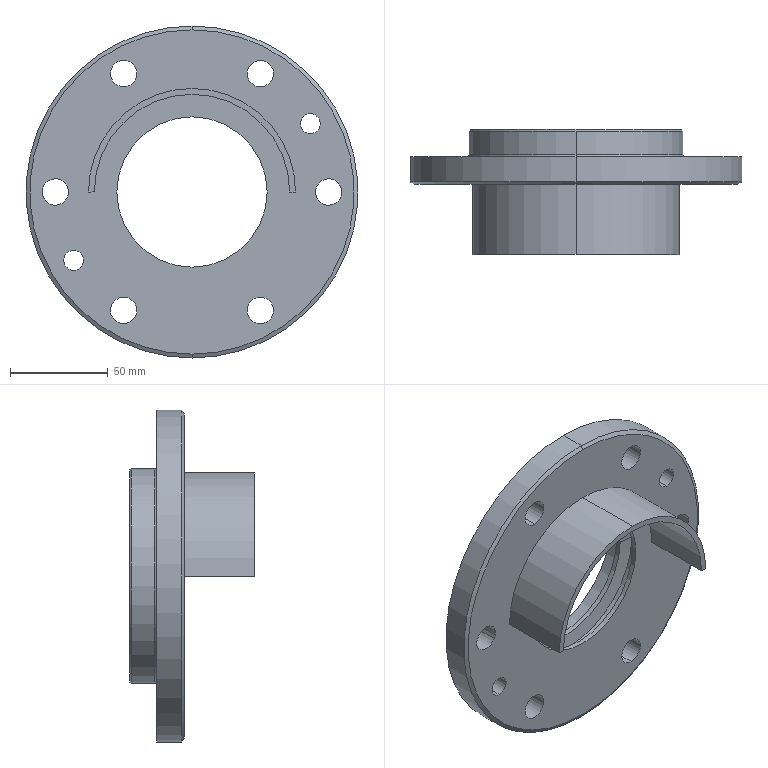Part | SolidWorks | features ICE 3, Chamfer 2, Fillet 2, CirPattern 1, Extrusion 1, HoleWzd 1, RevCut 1 | 1 solid | 51 faces | box 170 x 64 x 170 mm | volume 268447 mm3 | cylinder 32 | cone 8 | plane 7 | torus 4 | commonest cylinder face diameters 13.5 x12 10.2 x4 77 x4 92 x2 98 x2 100 x2
STEP:
#1=CARTESIAN_POINT('',(60.622,14.,29.9));
#2=VERTEX_POINT('',#1);
#3=CARTESIAN_POINT('',(60.622,14.,40.1));
#4=VERTEX_POINT('',#3);
#5=CARTESIAN_POINT('',(60.622,14.,35.));
#6=DIRECTION('',(0.,1.,0.));
#7=DIRECTION('',(0.,0.,1.));
#8=AXIS2_PLACEMENT_3D('',#5,#6,#7);
#9=CIRCLE('',#8,5.1);
#10=EDGE_CURVE('',#2,#4,#9,.T.);
#11=ORIENTED_EDGE('',*,*,#10,.T.);
#12=CARTESIAN_POINT('',(60.622,0.,40.1));
#13=VERTEX_POINT('',#12);
#14=CARTESIAN_POINT('',(60.622,0.,40.1));
#15=DIRECTION('',(0.,-1.,0.));
#16=VECTOR('',#15,1000.);
#17=LINE('',#14,#16);
#18=EDGE_CURVE('',#4,#13,#17,.T.);
#19=ORIENTED_EDGE('',*,*,#18,.T.);
#20=CARTESIAN_POINT('',(60.622,0.,29.9));
#21=VERTEX_POINT('',#20);
#22=CARTESIAN_POINT('',(60.622,0.,35.));
#23=DIRECTION('',(0.,-1.,0.));
#24=DIRECTION('',(0.,0.,-1.));
#25=AXIS2_PLACEMENT_3D('',#22,#23,#24);
#26=CIRCLE('',#25,5.1);
#27=EDGE_CURVE('',#13,#21,#26,.T.);
#28=ORIENTED_EDGE('',*,*,#27,.T.);
#29=CARTESIAN_POINT('',(60.622,0.,29.9));
#30=DIRECTION('',(0.,-1.,0.));
#31=VECTOR('',#30,1000.);
#32=LINE('',#29,#31);
#33=EDGE_CURVE('',#2,#21,#32,.T.);
#34=ORIENTED_EDGE('',*,*,#33,.F.);
#35=EDGE_LOOP('',(#11,#19,#28,#34));
#36=FACE_OUTER_BOUND('',#35,.T.);
#37=CARTESIAN_POINT('',(60.622,0.,35.));
#38=DIRECTION('',(0.,-1.,0.));
#39=DIRECTION('',(0.,0.,-1.));
#40=AXIS2_PLACEMENT_3D('',#37,#38,#39);
#41=CYLINDRICAL_SURFACE('',#40,5.1);
#42=ADVANCED_FACE('',(#36),#41,.F.);
#43=CARTESIAN_POINT('',(-60.622,14.,-40.1));
#44=VERTEX_POINT('',#43);
#45=CARTESIAN_POINT('',(-60.622,14.,-29.9));
#46=VERTEX_POINT('',#45);
#47=CARTESIAN_POINT('',(-60.622,14.,-35.));
#48=DIRECTION('',(0.,1.,0.));
#49=DIRECTION('',(0.,0.,1.));
#50=AXIS2_PLACEMENT_3D('',#47,#48,#49);
#51=CIRCLE('',#50,5.1);
#52=EDGE_CURVE('',#44,#46,#51,.T.);
#53=ORIENTED_EDGE('',*,*,#52,.T.);
#54=CARTESIAN_POINT('',(-60.622,0.,-29.9));
#55=VERTEX_POINT('',#54);
#56=CARTESIAN_POINT('',(-60.622,0.,-29.9));
#57=DIRECTION('',(0.,-1.,0.));
#58=VECTOR('',#57,1000.);
#59=LINE('',#56,#58);
#60=EDGE_CURVE('',#46,#55,#59,.T.);
#61=ORIENTED_EDGE('',*,*,#60,.T.);
#62=CARTESIAN_POINT('',(-60.622,0.,-40.1));
#63=VERTEX_POINT('',#62);
#64=CARTESIAN_POINT('',(-60.622,0.,-35.));
#65=DIRECTION('',(0.,-1.,0.));
#66=DIRECTION('',(0.,0.,-1.));
#67=AXIS2_PLACEMENT_3D('',#64,#65,#66);
#68=CIRCLE('',#67,5.1);
#69=EDGE_CURVE('',#55,#63,#68,.T.);
#70=ORIENTED_EDGE('',*,*,#69,.T.);
#71=CARTESIAN_POINT('',(-60.622,0.,-40.1));
#72=DIRECTION('',(0.,-1.,0.));
#73=VECTOR('',#72,1000.);
#74=LINE('',#71,#73);
#75=EDGE_CURVE('',#44,#63,#74,.T.);
#76=ORIENTED_EDGE('',*,*,#75,.F.);
#77=EDGE_LOOP('',(#53,#61,#70,#76));
#78=FACE_OUTER_BOUND('',#77,.T.);
#79=CARTESIAN_POINT('',(-60.622,0.,-35.));
#80=DIRECTION('',(0.,-1.,0.));
#81=DIRECTION('',(0.,0.,-1.));
#82=AXIS2_PLACEMENT_3D('',#79,#80,#81);
#83=CYLINDRICAL_SURFACE('',#82,5.1);
#84=ADVANCED_FACE('',(#78),#83,.F.);
#85=CARTESIAN_POINT('',(29.154,14.,57.247));
#86=VERTEX_POINT('',#85);
#87=CARTESIAN_POINT('',(40.846,14.,63.997));
#88=VERTEX_POINT('',#87);
#89=CARTESIAN_POINT('',(35.,14.,60.622));
#90=DIRECTION('',(0.,1.,0.));
#91=DIRECTION('',(0.866,0.,0.5));
#92=AXIS2_PLACEMENT_3D('',#89,#90,#91);
#93=CIRCLE('',#92,6.75);
#94=EDGE_CURVE('',#86,#88,#93,.T.);
#95=ORIENTED_EDGE('',*,*,#94,.T.);
#96=CARTESIAN_POINT('',(40.846,0.,63.997));
#97=VERTEX_POINT('',#96);
#98=CARTESIAN_POINT('',(40.846,28.,63.997));
#99=DIRECTION('',(0.,-1.,0.));
#100=VECTOR('',#99,1000.);
#101=LINE('',#98,#100);
#102=EDGE_CURVE('',#88,#97,#101,.T.);
#103=ORIENTED_EDGE('',*,*,#102,.T.);
#104=CARTESIAN_POINT('',(29.154,0.,57.247));
#105=VERTEX_POINT('',#104);
#106=CARTESIAN_POINT('',(35.,0.,60.622));
#107=DIRECTION('',(0.,-1.,0.));
#108=DIRECTION('',(-0.866,0.,-0.5));
#109=AXIS2_PLACEMENT_3D('',#106,#107,#108);
#110=CIRCLE('',#109,6.75);
#111=EDGE_CURVE('',#97,#105,#110,.T.);
#112=ORIENTED_EDGE('',*,*,#111,.T.);
#113=CARTESIAN_POINT('',(29.154,28.,57.247));
#114=DIRECTION('',(0.,-1.,0.));
#115=VECTOR('',#114,1000.);
#116=LINE('',#113,#115);
#117=EDGE_CURVE('',#86,#105,#116,.T.);
#118=ORIENTED_EDGE('',*,*,#117,.F.);
#119=EDGE_LOOP('',(#95,#103,#112,#118));
#120=FACE_OUTER_BOUND('',#119,.T.);
#121=CARTESIAN_POINT('',(35.,28.,60.622));
#122=DIRECTION('',(0.,-1.,0.));
#123=DIRECTION('',(-0.866,0.,-0.5));
#124=AXIS2_PLACEMENT_3D('',#121,#122,#123);
#125=CYLINDRICAL_SURFACE('',#124,6.75);
#126=ADVANCED_FACE('',(#120),#125,.F.);
#127=CARTESIAN_POINT('',(64.154,14.,3.375));
#128=VERTEX_POINT('',#127);
#129=CARTESIAN_POINT('',(75.846,14.,-3.375));
#130=VERTEX_POINT('',#129);
#131=CARTESIAN_POINT('',(70.,14.,0.));
#132=DIRECTION('',(0.,1.,0.));
#133=DIRECTION('',(0.866,0.,-0.5));
#134=AXIS2_PLACEMENT_3D('',#131,#132,#133);
#135=CIRCLE('',#134,6.75);
#136=EDGE_CURVE('',#128,#130,#135,.T.);
#137=ORIENTED_EDGE('',*,*,#136,.T.);
#138=CARTESIAN_POINT('',(75.846,0.,-3.375));
#139=VERTEX_POINT('',#138);
#140=CARTESIAN_POINT('',(75.846,28.,-3.375));
#141=DIRECTION('',(0.,-1.,0.));
#142=VECTOR('',#141,1000.);
#143=LINE('',#140,#142);
#144=EDGE_CURVE('',#130,#139,#143,.T.);
#145=ORIENTED_EDGE('',*,*,#144,.T.);
#146=CARTESIAN_POINT('',(64.154,0.,3.375));
#147=VERTEX_POINT('',#146);
#148=CARTESIAN_POINT('',(70.,0.,0.));
#149=DIRECTION('',(0.,-1.,0.));
#150=DIRECTION('',(-0.866,0.,0.5));
#151=AXIS2_PLACEMENT_3D('',#148,#149,#150);
#152=CIRCLE('',#151,6.75);
#153=EDGE_CURVE('',#139,#147,#152,.T.);
#154=ORIENTED_EDGE('',*,*,#153,.T.);
#155=CARTESIAN_POINT('',(64.154,28.,3.375));
#156=DIRECTION('',(0.,-1.,0.));
#157=VECTOR('',#156,1000.);
#158=LINE('',#155,#157);
#159=EDGE_CURVE('',#128,#147,#158,.T.);
#160=ORIENTED_EDGE('',*,*,#159,.F.);
#161=EDGE_LOOP('',(#137,#145,#154,#160));
#162=FACE_OUTER_BOUND('',#161,.T.);
#163=CARTESIAN_POINT('',(70.,28.,0.));
#164=DIRECTION('',(0.,-1.,0.));
#165=DIRECTION('',(-0.866,0.,0.5));
#166=AXIS2_PLACEMENT_3D('',#163,#164,#165);
#167=CYLINDRICAL_SURFACE('',#166,6.75);
#168=ADVANCED_FACE('',(#162),#167,.F.);
#169=CARTESIAN_POINT('',(35.,14.,-53.872));
#170=VERTEX_POINT('',#169);
#171=CARTESIAN_POINT('',(35.,14.,-67.372));
#172=VERTEX_POINT('',#171);
#173=CARTESIAN_POINT('',(35.,14.,-60.622));
#174=DIRECTION('',(0.,1.,0.));
#175=DIRECTION('',(0.,0.,-1.));
#176=AXIS2_PLACEMENT_3D('',#173,#174,#175);
#177=CIRCLE('',#176,6.75);
#178=EDGE_CURVE('',#170,#172,#177,.T.);
#179=ORIENTED_EDGE('',*,*,#178,.T.);
#180=CARTESIAN_POINT('',(35.,0.,-67.372));
#181=VERTEX_POINT('',#180);
#182=CARTESIAN_POINT('',(35.,28.,-67.372));
#183=DIRECTION('',(0.,-1.,0.));
#184=VECTOR('',#183,1000.);
#185=LINE('',#182,#184);
#186=EDGE_CURVE('',#172,#181,#185,.T.);
#187=ORIENTED_EDGE('',*,*,#186,.T.);
#188=CARTESIAN_POINT('',(35.,0.,-53.872));
#189=VERTEX_POINT('',#188);
#190=CARTESIAN_POINT('',(35.,0.,-60.622));
#191=DIRECTION('',(0.,-1.,0.));
#192=DIRECTION('',(0.,0.,1.));
#193=AXIS2_PLACEMENT_3D('',#190,#191,#192);
#194=CIRCLE('',#193,6.75);
#195=EDGE_CURVE('',#181,#189,#194,.T.);
#196=ORIENTED_EDGE('',*,*,#195,.T.);
#197=CARTESIAN_POINT('',(35.,28.,-53.872));
#198=DIRECTION('',(0.,-1.,0.));
#199=VECTOR('',#198,1000.);
#200=LINE('',#197,#199);
#201=EDGE_CURVE('',#170,#189,#200,.T.);
#202=ORIENTED_EDGE('',*,*,#201,.F.);
#203=EDGE_LOOP('',(#179,#187,#196,#202));
#204=FACE_OUTER_BOUND('',#203,.T.);
#205=CARTESIAN_POINT('',(35.,28.,-60.622));
#206=DIRECTION('',(0.,-1.,0.));
#207=DIRECTION('',(0.,0.,1.));
#208=AXIS2_PLACEMENT_3D('',#205,#206,#207);
#209=CYLINDRICAL_SURFACE('',#208,6.75);
#210=ADVANCED_FACE('',(#204),#209,.F.);
#211=CARTESIAN_POINT('',(-29.154,14.,-57.247));
#212=VERTEX_POINT('',#211);
#213=CARTESIAN_POINT('',(-40.846,14.,-63.997));
#214=VERTEX_POINT('',#213);
#215=CARTESIAN_POINT('',(-35.,14.,-60.622));
#216=DIRECTION('',(0.,1.,0.));
#217=DIRECTION('',(-0.866,0.,-0.5));
#218=AXIS2_PLACEMENT_3D('',#215,#216,#217);
#219=CIRCLE('',#218,6.75);
#220=EDGE_CURVE('',#212,#214,#219,.T.);
#221=ORIENTED_EDGE('',*,*,#220,.T.);
#222=CARTESIAN_POINT('',(-40.846,0.,-63.997));
#223=VERTEX_POINT('',#222);
#224=CARTESIAN_POINT('',(-40.846,28.,-63.997));
#225=DIRECTION('',(0.,-1.,0.));
#226=VECTOR('',#225,1000.);
#227=LINE('',#224,#226);
#228=EDGE_CURVE('',#214,#223,#227,.T.);
#229=ORIENTED_EDGE('',*,*,#228,.T.);
#230=CARTESIAN_POINT('',(-29.154,0.,-57.247));
#231=VERTEX_POINT('',#230);
#232=CARTESIAN_POINT('',(-35.,0.,-60.622));
#233=DIRECTION('',(0.,-1.,0.));
#234=DIRECTION('',(0.866,0.,0.5));
#235=AXIS2_PLACEMENT_3D('',#232,#233,#234);
#236=CIRCLE('',#235,6.75);
#237=EDGE_CURVE('',#223,#231,#236,.T.);
#238=ORIENTED_EDGE('',*,*,#237,.T.);
#239=CARTESIAN_POINT('',(-29.154,28.,-57.247));
#240=DIRECTION('',(0.,-1.,0.));
#241=VECTOR('',#240,1000.);
#242=LINE('',#239,#241);
#243=EDGE_CURVE('',#212,#231,#242,.T.);
#244=ORIENTED_EDGE('',*,*,#243,.F.);
#245=EDGE_LOOP('',(#221,#229,#238,#244));
#246=FACE_OUTER_BOUND('',#245,.T.);
#247=CARTESIAN_POINT('',(-35.,28.,-60.622));
#248=DIRECTION('',(0.,-1.,0.));
#249=DIRECTION('',(0.866,0.,0.5));
#250=AXIS2_PLACEMENT_3D('',#247,#248,#249);
#251=CYLINDRICAL_SURFACE('',#250,6.75);
#252=ADVANCED_FACE('',(#246),#251,.F.);
#253=CARTESIAN_POINT('',(-64.154,14.,-3.375));
#254=VERTEX_POINT('',#253);
#255=CARTESIAN_POINT('',(-75.846,14.,3.375));
#256=VERTEX_POINT('',#255);
#257=CARTESIAN_POINT('',(-70.,14.,0.));
#258=DIRECTION('',(0.,1.,0.));
#259=DIRECTION('',(-0.866,0.,0.5));
#260=AXIS2_PLACEMENT_3D('',#257,#258,#259);
#261=CIRCLE('',#260,6.75);
#262=EDGE_CURVE('',#254,#256,#261,.T.);
#263=ORIENTED_EDGE('',*,*,#262,.T.);
#264=CARTESIAN_POINT('',(-75.846,0.,3.375));
#265=VERTEX_POINT('',#264);
#266=CARTESIAN_POINT('',(-75.846,28.,3.375));
#267=DIRECTION('',(0.,-1.,0.));
#268=VECTOR('',#267,1000.);
#269=LINE('',#266,#268);
#270=EDGE_CURVE('',#256,#265,#269,.T.);
#271=ORIENTED_EDGE('',*,*,#270,.T.);
#272=CARTESIAN_POINT('',(-64.154,0.,-3.375));
#273=VERTEX_POINT('',#272);
#274=CARTESIAN_POINT('',(-70.,0.,0.));
#275=DIRECTION('',(0.,-1.,0.));
#276=DIRECTION('',(0.866,0.,-0.5));
#277=AXIS2_PLACEMENT_3D('',#274,#275,#276);
#278=CIRCLE('',#277,6.75);
#279=EDGE_CURVE('',#265,#273,#278,.T.);
#280=ORIENTED_EDGE('',*,*,#279,.T.);
#281=CARTESIAN_POINT('',(-64.154,28.,-3.375));
#282=DIRECTION('',(0.,-1.,0.));
#283=VECTOR('',#282,1000.);
#284=LINE('',#281,#283);
#285=EDGE_CURVE('',#254,#273,#284,.T.);
#286=ORIENTED_EDGE('',*,*,#285,.F.);
#287=EDGE_LOOP('',(#263,#271,#280,#286));
#288=FACE_OUTER_BOUND('',#287,.T.);
#289=CARTESIAN_POINT('',(-70.,28.,0.));
#290=DIRECTION('',(0.,-1.,0.));
#291=DIRECTION('',(0.866,0.,-0.5));
#292=AXIS2_PLACEMENT_3D('',#289,#290,#291);
#293=CYLINDRICAL_SURFACE('',#292,6.75);
#294=ADVANCED_FACE('',(#288),#293,.F.);
#295=CARTESIAN_POINT('',(-35.,14.,53.872));
#296=VERTEX_POINT('',#295);
#297=CARTESIAN_POINT('',(-35.,14.,67.372));
#298=VERTEX_POINT('',#297);
#299=CARTESIAN_POINT('',(-35.,14.,60.622));
#300=DIRECTION('',(0.,1.,0.));
#301=DIRECTION('',(0.,0.,1.));
#302=AXIS2_PLACEMENT_3D('',#299,#300,#301);
#303=CIRCLE('',#302,6.75);
#304=EDGE_CURVE('',#296,#298,#303,.T.);
#305=ORIENTED_EDGE('',*,*,#304,.T.);
#306=CARTESIAN_POINT('',(-35.,0.,67.372));
#307=VERTEX_POINT('',#306);
#308=CARTESIAN_POINT('',(-35.,28.,67.372));
#309=DIRECTION('',(0.,-1.,0.));
#310=VECTOR('',#309,1000.);
#311=LINE('',#308,#310);
#312=EDGE_CURVE('',#298,#307,#311,.T.);
#313=ORIENTED_EDGE('',*,*,#312,.T.);
#314=CARTESIAN_POINT('',(-35.,0.,53.872));
#315=VERTEX_POINT('',#314);
#316=CARTESIAN_POINT('',(-35.,0.,60.622));
#317=DIRECTION('',(0.,-1.,0.));
#318=DIRECTION('',(0.,0.,-1.));
#319=AXIS2_PLACEMENT_3D('',#316,#317,#318);
#320=CIRCLE('',#319,6.75);
#321=EDGE_CURVE('',#307,#315,#320,.T.);
#322=ORIENTED_EDGE('',*,*,#321,.T.);
#323=CARTESIAN_POINT('',(-35.,28.,53.872));
#324=DIRECTION('',(0.,-1.,0.));
#325=VECTOR('',#324,1000.);
#326=LINE('',#323,#325);
#327=EDGE_CURVE('',#296,#315,#326,.T.);
#328=ORIENTED_EDGE('',*,*,#327,.F.);
#329=EDGE_LOOP('',(#305,#313,#322,#328));
#330=FACE_OUTER_BOUND('',#329,.T.);
#331=CARTESIAN_POINT('',(-35.,28.,60.622));
#332=DIRECTION('',(0.,-1.,0.));
#333=DIRECTION('',(0.,0.,-1.));
#334=AXIS2_PLACEMENT_3D('',#331,#332,#333);
#335=CYLINDRICAL_SURFACE('',#334,6.75);
#336=ADVANCED_FACE('',(#330),#335,.F.);
#337=CARTESIAN_POINT('',(38.5,11.421,0.));
#338=VERTEX_POINT('',#337);
#339=CARTESIAN_POINT('',(-38.5,11.421,0.));
#340=VERTEX_POINT('',#339);
#341=CARTESIAN_POINT('',(0.,11.421,0.));
#342=DIRECTION('',(0.,1.,0.));
#343=DIRECTION('',(-1.,0.,0.));
#344=AXIS2_PLACEMENT_3D('',#341,#342,#343);
#345=CIRCLE('',#344,38.5);
#346=EDGE_CURVE('',#338,#340,#345,.T.);
#347=ORIENTED_EDGE('',*,*,#346,.F.);
#348=CARTESIAN_POINT('',(38.5,14.,0.));
#349=VERTEX_POINT('',#348);
#350=CARTESIAN_POINT('',(38.5,14.,0.));
#351=DIRECTION('',(0.,1.,0.));
#352=VECTOR('',#351,1000.);
#353=LINE('',#350,#352);
#354=EDGE_CURVE('',#338,#349,#353,.T.);
#355=ORIENTED_EDGE('',*,*,#354,.T.);
#356=CARTESIAN_POINT('',(-38.5,14.,0.));
#357=VERTEX_POINT('',#356);
#358=CARTESIAN_POINT('',(0.,14.,0.));
#359=DIRECTION('',(0.,1.,0.));
#360=DIRECTION('',(-1.,0.,0.));
#361=AXIS2_PLACEMENT_3D('',#358,#359,#360);
#362=CIRCLE('',#361,38.5);
#363=EDGE_CURVE('',#349,#357,#362,.T.);
#364=ORIENTED_EDGE('',*,*,#363,.T.);
#365=CARTESIAN_POINT('',(-38.5,14.,0.));
#366=DIRECTION('',(0.,1.,0.));
#367=VECTOR('',#366,1000.);
#368=LINE('',#365,#367);
#369=EDGE_CURVE('',#340,#357,#368,.T.);
#370=ORIENTED_EDGE('',*,*,#369,.F.);
#371=EDGE_LOOP('',(#347,#355,#364,#370));
#372=FACE_OUTER_BOUND('',#371,.T.);
#373=CARTESIAN_POINT('',(0.,14.,0.));
#374=DIRECTION('',(0.,1.,0.));
#375=DIRECTION('',(-1.,0.,0.));
#376=AXIS2_PLACEMENT_3D('',#373,#374,#375);
#377=CYLINDRICAL_SURFACE('',#376,38.5);
#378=ADVANCED_FACE('',(#372),#377,.F.);
#379=ORIENTED_EDGE('',*,*,#346,.T.);
#380=CARTESIAN_POINT('',(-46.,10.5,0.));
#381=VERTEX_POINT('',#380);
#382=CARTESIAN_POINT('',(-38.5,11.421,0.));
#383=DIRECTION('',(-0.9925,-0.1219,0.));
#384=VECTOR('',#383,1000.);
#385=LINE('',#382,#384);
#386=EDGE_CURVE('',#340,#381,#385,.T.);
#387=ORIENTED_EDGE('',*,*,#386,.T.);
#388=CARTESIAN_POINT('',(46.,10.5,0.));
#389=VERTEX_POINT('',#388);
#390=CARTESIAN_POINT('',(0.,10.5,0.));
#391=DIRECTION('',(0.,1.,0.));
#392=DIRECTION('',(-1.,0.,0.));
#393=AXIS2_PLACEMENT_3D('',#390,#391,#392);
#394=CIRCLE('',#393,46.);
#395=EDGE_CURVE('',#389,#381,#394,.T.);
#396=ORIENTED_EDGE('',*,*,#395,.F.);
#397=CARTESIAN_POINT('',(38.5,11.421,0.));
#398=DIRECTION('',(0.9925,-0.1219,0.));
#399=VECTOR('',#398,1000.);
#400=LINE('',#397,#399);
#401=EDGE_CURVE('',#338,#389,#400,.T.);
#402=ORIENTED_EDGE('',*,*,#401,.F.);
#403=EDGE_LOOP('',(#379,#387,#396,#402));
#404=FACE_OUTER_BOUND('',#403,.T.);
#405=CARTESIAN_POINT('',(0.,11.421,0.));
#406=DIRECTION('',(0.,-1.,0.));
#407=DIRECTION('',(1.,0.,0.));
#408=AXIS2_PLACEMENT_3D('',#405,#406,#407);
#409=CONICAL_SURFACE('',#408,38.5,1.449);
#410=ADVANCED_FACE('',(#404),#409,.F.);
#411=CARTESIAN_POINT('',(46.,3.5,0.));
#412=VERTEX_POINT('',#411);
#413=CARTESIAN_POINT('',(-46.,3.5,0.));
#414=VERTEX_POINT('',#413);
#415=CARTESIAN_POINT('',(0.,3.5,0.));
#416=DIRECTION('',(0.,1.,0.));
#417=DIRECTION('',(-1.,0.,0.));
#418=AXIS2_PLACEMENT_3D('',#415,#416,#417);
#419=CIRCLE('',#418,46.);
#420=EDGE_CURVE('',#412,#414,#419,.T.);
#421=ORIENTED_EDGE('',*,*,#420,.F.);
#422=CARTESIAN_POINT('',(46.,14.,0.));
#423=DIRECTION('',(0.,1.,0.));
#424=VECTOR('',#423,1000.);
#425=LINE('',#422,#424);
#426=EDGE_CURVE('',#412,#389,#425,.T.);
#427=ORIENTED_EDGE('',*,*,#426,.T.);
#428=ORIENTED_EDGE('',*,*,#395,.T.);
#429=CARTESIAN_POINT('',(-46.,14.,0.));
#430=DIRECTION('',(0.,1.,0.));
#431=VECTOR('',#430,1000.);
#432=LINE('',#429,#431);
#433=EDGE_CURVE('',#414,#381,#432,.T.);
#434=ORIENTED_EDGE('',*,*,#433,.F.);
#435=EDGE_LOOP('',(#421,#427,#428,#434));
#436=FACE_OUTER_BOUND('',#435,.T.);
#437=CARTESIAN_POINT('',(0.,14.,0.));
#438=DIRECTION('',(0.,1.,0.));
#439=DIRECTION('',(-1.,0.,0.));
#440=AXIS2_PLACEMENT_3D('',#437,#438,#439);
#441=CYLINDRICAL_SURFACE('',#440,46.);
#442=ADVANCED_FACE('',(#436),#441,.F.);
#443=CARTESIAN_POINT('',(38.5,2.579,0.));
#444=VERTEX_POINT('',#443);
#445=CARTESIAN_POINT('',(-38.5,2.579,0.));
#446=VERTEX_POINT('',#445);
#447=CARTESIAN_POINT('',(0.,2.579,0.));
#448=DIRECTION('',(0.,1.,0.));
#449=DIRECTION('',(-1.,0.,0.));
#450=AXIS2_PLACEMENT_3D('',#447,#448,#449);
#451=CIRCLE('',#450,38.5);
#452=EDGE_CURVE('',#444,#446,#451,.T.);
#453=ORIENTED_EDGE('',*,*,#452,.F.);
#454=CARTESIAN_POINT('',(46.,3.5,0.));
#455=DIRECTION('',(0.9925,0.1219,0.));
#456=VECTOR('',#455,1000.);
#457=LINE('',#454,#456);
#458=EDGE_CURVE('',#444,#412,#457,.T.);
#459=ORIENTED_EDGE('',*,*,#458,.T.);
#460=ORIENTED_EDGE('',*,*,#420,.T.);
#461=CARTESIAN_POINT('',(-46.,3.5,0.));
#462=DIRECTION('',(-0.9925,0.1219,0.));
#463=VECTOR('',#462,1000.);
#464=LINE('',#461,#463);
#465=EDGE_CURVE('',#446,#414,#464,.T.);
#466=ORIENTED_EDGE('',*,*,#465,.F.);
#467=EDGE_LOOP('',(#453,#459,#460,#466));
#468=FACE_OUTER_BOUND('',#467,.T.);
#469=CARTESIAN_POINT('',(0.,3.5,0.));
#470=DIRECTION('',(0.,1.,0.));
#471=DIRECTION('',(-1.,0.,0.));
#472=AXIS2_PLACEMENT_3D('',#469,#470,#471);
#473=CONICAL_SURFACE('',#472,46.,1.449);
#474=ADVANCED_FACE('',(#468),#473,.F.);
#475=CARTESIAN_POINT('',(38.5,0.,0.));
#476=VERTEX_POINT('',#475);
#477=CARTESIAN_POINT('',(-38.5,0.,0.));
#478=VERTEX_POINT('',#477);
#479=CARTESIAN_POINT('',(0.,0.,0.));
#480=DIRECTION('',(0.,1.,0.));
#481=DIRECTION('',(-1.,0.,0.));
#482=AXIS2_PLACEMENT_3D('',#479,#480,#481);
#483=CIRCLE('',#482,38.5);
#484=EDGE_CURVE('',#476,#478,#483,.T.);
#485=ORIENTED_EDGE('',*,*,#484,.F.);
#486=CARTESIAN_POINT('',(38.5,14.,0.));
#487=DIRECTION('',(0.,1.,0.));
#488=VECTOR('',#487,1000.);
#489=LINE('',#486,#488);
#490=EDGE_CURVE('',#476,#444,#489,.T.);
#491=ORIENTED_EDGE('',*,*,#490,.T.);
#492=ORIENTED_EDGE('',*,*,#452,.T.);
#493=CARTESIAN_POINT('',(-38.5,14.,0.));
#494=DIRECTION('',(0.,1.,0.));
#495=VECTOR('',#494,1000.);
#496=LINE('',#493,#495);
#497=EDGE_CURVE('',#478,#446,#496,.T.);
#498=ORIENTED_EDGE('',*,*,#497,.F.);
#499=EDGE_LOOP('',(#485,#491,#492,#498));
#500=FACE_OUTER_BOUND('',#499,.T.);
#501=CARTESIAN_POINT('',(0.,14.,0.));
#502=DIRECTION('',(0.,1.,0.));
#503=DIRECTION('',(-1.,0.,0.));
#504=AXIS2_PLACEMENT_3D('',#501,#502,#503);
#505=CYLINDRICAL_SURFACE('',#504,38.5);
#506=ADVANCED_FACE('',(#500),#505,.F.);
#507=CARTESIAN_POINT('',(0.,-36.,50.));
#508=VERTEX_POINT('',#507);
#509=CARTESIAN_POINT('',(50.,-36.,0.));
#510=VERTEX_POINT('',#509);
#511=CARTESIAN_POINT('',(0.,-36.,0.));
#512=DIRECTION('',(0.,1.,0.));
#513=DIRECTION('',(0.,0.,-1.));
#514=AXIS2_PLACEMENT_3D('',#511,#512,#513);
#515=CIRCLE('',#514,50.);
#516=EDGE_CURVE('',#508,#510,#515,.T.);
#517=ORIENTED_EDGE('',*,*,#516,.F.);
#518=CARTESIAN_POINT('',(0.,0.,50.));
#519=VERTEX_POINT('',#518);
#520=CARTESIAN_POINT('',(0.,-36.,50.));
#521=DIRECTION('',(0.,1.,0.));
#522=VECTOR('',#521,1000.);
#523=LINE('',#520,#522);
#524=EDGE_CURVE('',#508,#519,#523,.T.);
#525=ORIENTED_EDGE('',*,*,#524,.T.);
#526=CARTESIAN_POINT('',(50.,0.,0.));
#527=VERTEX_POINT('',#526);
#528=CARTESIAN_POINT('',(0.,0.,0.));
#529=DIRECTION('',(0.,1.,0.));
#530=DIRECTION('',(0.,0.,-1.));
#531=AXIS2_PLACEMENT_3D('',#528,#529,#530);
#532=CIRCLE('',#531,50.);
#533=EDGE_CURVE('',#519,#527,#532,.T.);
#534=ORIENTED_EDGE('',*,*,#533,.T.);
#535=CARTESIAN_POINT('',(50.,-36.,0.));
#536=DIRECTION('',(0.,1.,0.));
#537=VECTOR('',#536,1000.);
#538=LINE('',#535,#537);
#539=EDGE_CURVE('',#510,#527,#538,.T.);
#540=ORIENTED_EDGE('',*,*,#539,.F.);
#541=EDGE_LOOP('',(#517,#525,#534,#540));
#542=FACE_OUTER_BOUND('',#541,.T.);
#543=CARTESIAN_POINT('',(0.,-36.,0.));
#544=DIRECTION('',(0.,1.,0.));
#545=DIRECTION('',(0.,0.,1.));
#546=AXIS2_PLACEMENT_3D('',#543,#544,#545);
#547=CYLINDRICAL_SURFACE('',#546,50.);
#548=ADVANCED_FACE('',(#542),#547,.F.);
#549=CARTESIAN_POINT('',(0.,-36.,53.));
#550=VERTEX_POINT('',#549);
#551=CARTESIAN_POINT('',(-53.,-36.,0.));
#552=VERTEX_POINT('',#551);
#553=CARTESIAN_POINT('',(0.,-36.,0.));
#554=DIRECTION('',(0.,-1.,0.));
#555=DIRECTION('',(0.,0.,-1.));
#556=AXIS2_PLACEMENT_3D('',#553,#554,#555);
#557=CIRCLE('',#556,53.);
#558=EDGE_CURVE('',#550,#552,#557,.T.);
#559=ORIENTED_EDGE('',*,*,#558,.F.);
#560=CARTESIAN_POINT('',(0.,0.,53.));
#561=VERTEX_POINT('',#560);
#562=CARTESIAN_POINT('',(0.,-36.,53.));
#563=DIRECTION('',(0.,1.,0.));
#564=VECTOR('',#563,1000.);
#565=LINE('',#562,#564);
#566=EDGE_CURVE('',#550,#561,#565,.T.);
#567=ORIENTED_EDGE('',*,*,#566,.T.);
#568=CARTESIAN_POINT('',(-53.,0.,0.));
#569=VERTEX_POINT('',#568);
#570=CARTESIAN_POINT('',(0.,0.,0.));
#571=DIRECTION('',(0.,-1.,0.));
#572=DIRECTION('',(0.,0.,-1.));
#573=AXIS2_PLACEMENT_3D('',#570,#571,#572);
#574=CIRCLE('',#573,53.);
#575=EDGE_CURVE('',#561,#569,#574,.T.);
#576=ORIENTED_EDGE('',*,*,#575,.T.);
#577=CARTESIAN_POINT('',(-53.,-36.,0.));
#578=DIRECTION('',(0.,1.,0.));
#579=VECTOR('',#578,1000.);
#580=LINE('',#577,#579);
#581=EDGE_CURVE('',#552,#569,#580,.T.);
#582=ORIENTED_EDGE('',*,*,#581,.F.);
#583=EDGE_LOOP('',(#559,#567,#576,#582));
#584=FACE_OUTER_BOUND('',#583,.T.);
#585=CARTESIAN_POINT('',(0.,-36.,0.));
#586=DIRECTION('',(0.,1.,0.));
#587=DIRECTION('',(0.,0.,1.));
#588=AXIS2_PLACEMENT_3D('',#585,#586,#587);
#589=CYLINDRICAL_SURFACE('',#588,53.);
#590=ADVANCED_FACE('',(#584),#589,.T.);
#591=CARTESIAN_POINT('',(0.,28.,54.423));
#592=VERTEX_POINT('',#591);
#593=CARTESIAN_POINT('',(0.,28.,-54.423));
#594=VERTEX_POINT('',#593);
#595=CARTESIAN_POINT('',(0.,28.,0.));
#596=DIRECTION('',(0.,1.,0.));
#597=DIRECTION('',(0.,0.,1.));
#598=AXIS2_PLACEMENT_3D('',#595,#596,#597);
#599=CIRCLE('',#598,54.423);
#600=EDGE_CURVE('',#592,#594,#599,.T.);
#601=ORIENTED_EDGE('',*,*,#600,.F.);
#602=CARTESIAN_POINT('',(0.,27.,55.));
#603=VERTEX_POINT('',#602);
#604=CARTESIAN_POINT('',(0.,28.,54.423));
#605=DIRECTION('',(0.,-0.866,0.5));
#606=VECTOR('',#605,1000.);
#607=LINE('',#604,#606);
#608=EDGE_CURVE('',#592,#603,#607,.T.);
#609=ORIENTED_EDGE('',*,*,#608,.T.);
#610=CARTESIAN_POINT('',(0.,27.,-55.));
#611=VERTEX_POINT('',#610);
#612=CARTESIAN_POINT('',(0.,27.,0.));
#613=DIRECTION('',(0.,-1.,0.));
#614=DIRECTION('',(0.,0.,1.));
#615=AXIS2_PLACEMENT_3D('',#612,#613,#614);
#616=CIRCLE('',#615,55.);
#617=EDGE_CURVE('',#611,#603,#616,.T.);
#618=ORIENTED_EDGE('',*,*,#617,.F.);
#619=CARTESIAN_POINT('',(0.,28.,-54.423));
#620=DIRECTION('',(0.,-0.866,-0.5));
#621=VECTOR('',#620,1000.);
#622=LINE('',#619,#621);
#623=EDGE_CURVE('',#594,#611,#622,.T.);
#624=ORIENTED_EDGE('',*,*,#623,.F.);
#625=EDGE_LOOP('',(#601,#609,#618,#624));
#626=FACE_OUTER_BOUND('',#625,.T.);
#627=CARTESIAN_POINT('',(0.,28.,0.));
#628=DIRECTION('',(0.,-1.,0.));
#629=DIRECTION('',(0.,0.,-1.));
#630=AXIS2_PLACEMENT_3D('',#627,#628,#629);
#631=CONICAL_SURFACE('',#630,54.423,0.5236);
#632=ADVANCED_FACE('',(#626),#631,.T.);
#633=CARTESIAN_POINT('',(0.,0.,-83.));
#634=VERTEX_POINT('',#633);
#635=CARTESIAN_POINT('',(0.,0.,83.));
#636=VERTEX_POINT('',#635);
#637=CARTESIAN_POINT('',(0.,0.,0.));
#638=DIRECTION('',(0.,-1.,0.));
#639=DIRECTION('',(0.,0.,1.));
#640=AXIS2_PLACEMENT_3D('',#637,#638,#639);
#641=CIRCLE('',#640,83.);
#642=EDGE_CURVE('',#634,#636,#641,.T.);
#643=ORIENTED_EDGE('',*,*,#642,.F.);
#644=CARTESIAN_POINT('',(0.,1.155,-85.));
#645=VERTEX_POINT('',#644);
#646=CARTESIAN_POINT('',(0.,1.155,-85.));
#647=DIRECTION('',(0.,0.5,-0.866));
#648=VECTOR('',#647,1000.);
#649=LINE('',#646,#648);
#650=EDGE_CURVE('',#634,#645,#649,.T.);
#651=ORIENTED_EDGE('',*,*,#650,.T.);
#652=CARTESIAN_POINT('',(0.,1.155,85.));
#653=VERTEX_POINT('',#652);
#654=CARTESIAN_POINT('',(0.,1.155,0.));
#655=DIRECTION('',(0.,1.,0.));
#656=DIRECTION('',(0.,0.,1.));
#657=AXIS2_PLACEMENT_3D('',#654,#655,#656);
#658=CIRCLE('',#657,85.);
#659=EDGE_CURVE('',#653,#645,#658,.T.);
#660=ORIENTED_EDGE('',*,*,#659,.F.);
#661=CARTESIAN_POINT('',(0.,1.155,85.));
#662=DIRECTION('',(0.,0.5,0.866));
#663=VECTOR('',#662,1000.);
#664=LINE('',#661,#663);
#665=EDGE_CURVE('',#636,#653,#664,.T.);
#666=ORIENTED_EDGE('',*,*,#665,.F.);
#667=EDGE_LOOP('',(#643,#651,#660,#666));
#668=FACE_OUTER_BOUND('',#667,.T.);
#669=CARTESIAN_POINT('',(0.,1.155,0.));
#670=DIRECTION('',(0.,1.,0.));
#671=DIRECTION('',(0.,0.,1.));
#672=AXIS2_PLACEMENT_3D('',#669,#670,#671);
#673=CONICAL_SURFACE('',#672,85.,1.047);
#674=ADVANCED_FACE('',(#668),#673,.T.);
#675=CARTESIAN_POINT('',(0.,15.,-55.));
#676=VERTEX_POINT('',#675);
#677=CARTESIAN_POINT('',(0.,15.,55.));
#678=VERTEX_POINT('',#677);
#679=CARTESIAN_POINT('',(0.,15.,0.));
#680=DIRECTION('',(0.,1.,0.));
#681=DIRECTION('',(0.,0.,1.));
#682=AXIS2_PLACEMENT_3D('',#679,#680,#681);
#683=CIRCLE('',#682,55.);
#684=EDGE_CURVE('',#676,#678,#683,.T.);
#685=ORIENTED_EDGE('',*,*,#684,.F.);
#686=CARTESIAN_POINT('',(0.,14.,-56.));
#687=VERTEX_POINT('',#686);
#688=CARTESIAN_POINT('',(0.,15.,-56.));
#689=DIRECTION('',(1.,0.,0.));
#690=DIRECTION('',(0.,0.,-1.));
#691=AXIS2_PLACEMENT_3D('',#688,#689,#690);
#692=CIRCLE('',#691,1.);
#693=EDGE_CURVE('',#676,#687,#692,.T.);
#694=ORIENTED_EDGE('',*,*,#693,.T.);
#695=CARTESIAN_POINT('',(0.,14.,56.));
#696=VERTEX_POINT('',#695);
#697=CARTESIAN_POINT('',(0.,14.,0.));
#698=DIRECTION('',(0.,-1.,0.));
#699=DIRECTION('',(0.,0.,1.));
#700=AXIS2_PLACEMENT_3D('',#697,#698,#699);
#701=CIRCLE('',#700,56.);
#702=EDGE_CURVE('',#696,#687,#701,.T.);
#703=ORIENTED_EDGE('',*,*,#702,.F.);
#704=CARTESIAN_POINT('',(0.,15.,56.));
#705=DIRECTION('',(-1.,0.,0.));
#706=DIRECTION('',(0.,0.,1.));
#707=AXIS2_PLACEMENT_3D('',#704,#705,#706);
#708=CIRCLE('',#707,1.);
#709=EDGE_CURVE('',#678,#696,#708,.T.);
#710=ORIENTED_EDGE('',*,*,#709,.F.);
#711=EDGE_LOOP('',(#685,#694,#703,#710));
#712=FACE_OUTER_BOUND('',#711,.T.);
#713=CARTESIAN_POINT('',(0.,15.,0.));
#714=DIRECTION('',(0.,1.,0.));
#715=DIRECTION('',(0.,0.,1.));
#716=AXIS2_PLACEMENT_3D('',#713,#714,#715);
#717=TOROIDAL_SURFACE('',#716,56.,1.);
#718=ADVANCED_FACE('',(#712),#717,.F.);
#719=CARTESIAN_POINT('',(0.,14.,-44.));
#720=VERTEX_POINT('',#719);
#721=CARTESIAN_POINT('',(0.,14.,44.));
#722=VERTEX_POINT('',#721);
#723=CARTESIAN_POINT('',(0.,14.,0.));
#724=DIRECTION('',(0.,1.,0.));
#725=DIRECTION('',(0.,0.,1.));
#726=AXIS2_PLACEMENT_3D('',#723,#724,#725);
#727=CIRCLE('',#726,44.);
#728=EDGE_CURVE('',#720,#722,#727,.T.);
#729=ORIENTED_EDGE('',*,*,#728,.F.);
#730=CARTESIAN_POINT('',(0.,19.,-49.));
#731=VERTEX_POINT('',#730);
#732=CARTESIAN_POINT('',(0.,19.,-44.));
#733=DIRECTION('',(1.,0.,0.));
#734=DIRECTION('',(0.,0.,-1.));
#735=AXIS2_PLACEMENT_3D('',#732,#733,#734);
#736=CIRCLE('',#735,5.);
#737=EDGE_CURVE('',#720,#731,#736,.T.);
#738=ORIENTED_EDGE('',*,*,#737,.T.);
#739=CARTESIAN_POINT('',(0.,19.,49.));
#740=VERTEX_POINT('',#739);
#741=CARTESIAN_POINT('',(0.,19.,0.));
#742=DIRECTION('',(0.,-1.,0.));
#743=DIRECTION('',(0.,0.,1.));
#744=AXIS2_PLACEMENT_3D('',#741,#742,#743);
#745=CIRCLE('',#744,49.);
#746=EDGE_CURVE('',#740,#731,#745,.T.);
#747=ORIENTED_EDGE('',*,*,#746,.F.);
#748=CARTESIAN_POINT('',(0.,19.,44.));
#749=DIRECTION('',(-1.,0.,0.));
#750=DIRECTION('',(0.,0.,1.));
#751=AXIS2_PLACEMENT_3D('',#748,#749,#750);
#752=CIRCLE('',#751,5.);
#753=EDGE_CURVE('',#722,#740,#752,.T.);
#754=ORIENTED_EDGE('',*,*,#753,.F.);
#755=EDGE_LOOP('',(#729,#738,#747,#754));
#756=FACE_OUTER_BOUND('',#755,.T.);
#757=CARTESIAN_POINT('',(0.,19.,0.));
#758=DIRECTION('',(0.,1.,0.));
#759=DIRECTION('',(0.,0.,1.));
#760=AXIS2_PLACEMENT_3D('',#757,#758,#759);
#761=TOROIDAL_SURFACE('',#760,44.,5.);
#762=ADVANCED_FACE('',(#756),#761,.F.);
#763=CARTESIAN_POINT('',(0.,28.,-49.));
#764=VERTEX_POINT('',#763);
#765=CARTESIAN_POINT('',(0.,28.,49.));
#766=VERTEX_POINT('',#765);
#767=CARTESIAN_POINT('',(0.,28.,0.));
#768=DIRECTION('',(0.,1.,0.));
#769=DIRECTION('',(0.,0.,1.));
#770=AXIS2_PLACEMENT_3D('',#767,#768,#769);
#771=CIRCLE('',#770,49.);
#772=EDGE_CURVE('',#764,#766,#771,.T.);
#773=ORIENTED_EDGE('',*,*,#772,.T.);
#774=CARTESIAN_POINT('',(0.,28.,49.));
#775=DIRECTION('',(0.,-1.,0.));
#776=VECTOR('',#775,1000.);
#777=LINE('',#774,#776);
#778=EDGE_CURVE('',#766,#740,#777,.T.);
#779=ORIENTED_EDGE('',*,*,#778,.T.);
#780=ORIENTED_EDGE('',*,*,#746,.T.);
#781=CARTESIAN_POINT('',(0.,28.,-49.));
#782=DIRECTION('',(0.,-1.,0.));
#783=VECTOR('',#782,1000.);
#784=LINE('',#781,#783);
#785=EDGE_CURVE('',#764,#731,#784,.T.);
#786=ORIENTED_EDGE('',*,*,#785,.F.);
#787=EDGE_LOOP('',(#773,#779,#780,#786));
#788=FACE_OUTER_BOUND('',#787,.T.);
#789=CARTESIAN_POINT('',(0.,28.,0.));
#790=DIRECTION('',(0.,-1.,0.));
#791=DIRECTION('',(0.,0.,-1.));
#792=AXIS2_PLACEMENT_3D('',#789,#790,#791);
#793=CYLINDRICAL_SURFACE('',#792,49.);
#794=ADVANCED_FACE('',(#788),#793,.F.);
#795=ORIENTED_EDGE('',*,*,#617,.T.);
#796=CARTESIAN_POINT('',(0.,28.,55.));
#797=DIRECTION('',(0.,-1.,0.));
#798=VECTOR('',#797,1000.);
#799=LINE('',#796,#798);
#800=EDGE_CURVE('',#603,#678,#799,.T.);
#801=ORIENTED_EDGE('',*,*,#800,.T.);
#802=CARTESIAN_POINT('',(0.,15.,0.));
#803=DIRECTION('',(0.,1.,0.));
#804=DIRECTION('',(0.,0.,1.));
#805=AXIS2_PLACEMENT_3D('',#802,#803,#804);
#806=CIRCLE('',#805,55.);
#807=EDGE_CURVE('',#678,#676,#806,.T.);
#808=ORIENTED_EDGE('',*,*,#807,.T.);
#809=CARTESIAN_POINT('',(0.,28.,-55.));
#810=DIRECTION('',(0.,-1.,0.));
#811=VECTOR('',#810,1000.);
#812=LINE('',#809,#811);
#813=EDGE_CURVE('',#611,#676,#812,.T.);
#814=ORIENTED_EDGE('',*,*,#813,.F.);
#815=EDGE_LOOP('',(#795,#801,#808,#814));
#816=FACE_OUTER_BOUND('',#815,.T.);
#817=CARTESIAN_POINT('',(0.,28.,0.));
#818=DIRECTION('',(0.,-1.,0.));
#819=DIRECTION('',(0.,0.,-1.));
#820=AXIS2_PLACEMENT_3D('',#817,#818,#819);
#821=CYLINDRICAL_SURFACE('',#820,55.);
#822=ADVANCED_FACE('',(#816),#821,.T.);
#823=CARTESIAN_POINT('',(0.,14.,85.));
#824=VERTEX_POINT('',#823);
#825=CARTESIAN_POINT('',(0.,14.,-85.));
#826=VERTEX_POINT('',#825);
#827=CARTESIAN_POINT('',(0.,14.,0.));
#828=DIRECTION('',(0.,1.,0.));
#829=DIRECTION('',(0.,0.,1.));
#830=AXIS2_PLACEMENT_3D('',#827,#828,#829);
#831=CIRCLE('',#830,85.);
#832=EDGE_CURVE('',#824,#826,#831,.T.);
#833=ORIENTED_EDGE('',*,*,#832,.F.);
#834=CARTESIAN_POINT('',(0.,14.,85.));
#835=DIRECTION('',(0.,-1.,0.));
#836=VECTOR('',#835,1000.);
#837=LINE('',#834,#836);
#838=EDGE_CURVE('',#824,#653,#837,.T.);
#839=ORIENTED_EDGE('',*,*,#838,.T.);
#840=ORIENTED_EDGE('',*,*,#659,.T.);
#841=CARTESIAN_POINT('',(0.,14.,-85.));
#842=DIRECTION('',(0.,-1.,0.));
#843=VECTOR('',#842,1000.);
#844=LINE('',#841,#843);
#845=EDGE_CURVE('',#826,#645,#844,.T.);
#846=ORIENTED_EDGE('',*,*,#845,.F.);
#847=EDGE_LOOP('',(#833,#839,#840,#846));
#848=FACE_OUTER_BOUND('',#847,.T.);
#849=CARTESIAN_POINT('',(0.,14.,0.));
#850=DIRECTION('',(0.,-1.,0.));
#851=DIRECTION('',(0.,0.,-1.));
#852=AXIS2_PLACEMENT_3D('',#849,#850,#851);
#853=CYLINDRICAL_SURFACE('',#852,85.);
#854=ADVANCED_FACE('',(#848),#853,.T.);
#855=CARTESIAN_POINT('',(60.622,0.,35.));
#856=DIRECTION('',(0.,-1.,0.));
#857=DIRECTION('',(0.,0.,-1.));
#858=AXIS2_PLACEMENT_3D('',#855,#856,#857);
#859=CIRCLE('',#858,5.1);
#860=EDGE_CURVE('',#21,#13,#859,.T.);
#861=ORIENTED_EDGE('',*,*,#860,.F.);
#862=ORIENTED_EDGE('',*,*,#27,.F.);
#863=EDGE_LOOP('',(#861,#862));
#864=FACE_BOUND('',#863,.T.);
#865=CARTESIAN_POINT('',(-60.622,0.,-35.));
#866=DIRECTION('',(0.,-1.,0.));
#867=DIRECTION('',(0.,0.,-1.));
#868=AXIS2_PLACEMENT_3D('',#865,#866,#867);
#869=CIRCLE('',#868,5.1);
#870=EDGE_CURVE('',#63,#55,#869,.T.);
#871=ORIENTED_EDGE('',*,*,#870,.F.);
#872=ORIENTED_EDGE('',*,*,#69,.F.);
#873=EDGE_LOOP('',(#871,#872));
#874=FACE_BOUND('',#873,.T.);
#875=CARTESIAN_POINT('',(35.,0.,60.622));
#876=DIRECTION('',(0.,-1.,0.));
#877=DIRECTION('',(-0.866,0.,-0.5));
#878=AXIS2_PLACEMENT_3D('',#875,#876,#877);
#879=CIRCLE('',#878,6.75);
#880=EDGE_CURVE('',#105,#97,#879,.T.);
#881=ORIENTED_EDGE('',*,*,#880,.F.);
#882=ORIENTED_EDGE('',*,*,#111,.F.);
#883=EDGE_LOOP('',(#881,#882));
#884=FACE_BOUND('',#883,.T.);
#885=CARTESIAN_POINT('',(70.,0.,0.));
#886=DIRECTION('',(0.,-1.,0.));
#887=DIRECTION('',(-0.866,0.,0.5));
#888=AXIS2_PLACEMENT_3D('',#885,#886,#887);
#889=CIRCLE('',#888,6.75);
#890=EDGE_CURVE('',#147,#139,#889,.T.);
#891=ORIENTED_EDGE('',*,*,#890,.F.);
#892=ORIENTED_EDGE('',*,*,#153,.F.);
#893=EDGE_LOOP('',(#891,#892));
#894=FACE_BOUND('',#893,.T.);
#895=CARTESIAN_POINT('',(35.,0.,-60.622));
#896=DIRECTION('',(0.,-1.,0.));
#897=DIRECTION('',(0.,0.,1.));
#898=AXIS2_PLACEMENT_3D('',#895,#896,#897);
#899=CIRCLE('',#898,6.75);
#900=EDGE_CURVE('',#189,#181,#899,.T.);
#901=ORIENTED_EDGE('',*,*,#900,.F.);
#902=ORIENTED_EDGE('',*,*,#195,.F.);
#903=EDGE_LOOP('',(#901,#902));
#904=FACE_BOUND('',#903,.T.);
#905=CARTESIAN_POINT('',(-35.,0.,-60.622));
#906=DIRECTION('',(0.,-1.,0.));
#907=DIRECTION('',(0.866,0.,0.5));
#908=AXIS2_PLACEMENT_3D('',#905,#906,#907);
#909=CIRCLE('',#908,6.75);
#910=EDGE_CURVE('',#231,#223,#909,.T.);
#911=ORIENTED_EDGE('',*,*,#910,.F.);
#912=ORIENTED_EDGE('',*,*,#237,.F.);
#913=EDGE_LOOP('',(#911,#912));
#914=FACE_BOUND('',#913,.T.);
#915=CARTESIAN_POINT('',(-70.,0.,0.));
#916=DIRECTION('',(0.,-1.,0.));
#917=DIRECTION('',(0.866,0.,-0.5));
#918=AXIS2_PLACEMENT_3D('',#915,#916,#917);
#919=CIRCLE('',#918,6.75);
#920=EDGE_CURVE('',#273,#265,#919,.T.);
#921=ORIENTED_EDGE('',*,*,#920,.F.);
#922=ORIENTED_EDGE('',*,*,#279,.F.);
#923=EDGE_LOOP('',(#921,#922));
#924=FACE_BOUND('',#923,.T.);
#925=CARTESIAN_POINT('',(-35.,0.,60.622));
#926=DIRECTION('',(0.,-1.,0.));
#927=DIRECTION('',(0.,0.,-1.));
#928=AXIS2_PLACEMENT_3D('',#925,#926,#927);
#929=CIRCLE('',#928,6.75);
#930=EDGE_CURVE('',#315,#307,#929,.T.);
#931=ORIENTED_EDGE('',*,*,#930,.F.);
#932=ORIENTED_EDGE('',*,*,#321,.F.);
#933=EDGE_LOOP('',(#931,#932));
#934=FACE_BOUND('',#933,.T.);
#935=CARTESIAN_POINT('',(0.,0.,0.));
#936=DIRECTION('',(0.,1.,0.));
#937=DIRECTION('',(-1.,0.,0.));
#938=AXIS2_PLACEMENT_3D('',#935,#936,#937);
#939=CIRCLE('',#938,38.5);
#940=EDGE_CURVE('',#478,#476,#939,.T.);
#941=ORIENTED_EDGE('',*,*,#940,.T.);
#942=ORIENTED_EDGE('',*,*,#484,.T.);
#943=EDGE_LOOP('',(#941,#942));
#944=FACE_BOUND('',#943,.T.);
#945=CARTESIAN_POINT('',(0.,0.,0.));
#946=DIRECTION('',(0.,-1.,0.));
#947=DIRECTION('',(0.,0.,1.));
#948=AXIS2_PLACEMENT_3D('',#945,#946,#947);
#949=CIRCLE('',#948,83.);
#950=EDGE_CURVE('',#636,#634,#949,.T.);
#951=ORIENTED_EDGE('',*,*,#950,.T.);
#952=ORIENTED_EDGE('',*,*,#642,.T.);
#953=EDGE_LOOP('',(#951,#952));
#954=FACE_OUTER_BOUND('',#953,.T.);
#955=CARTESIAN_POINT('',(53.,0.,0.));
#956=VERTEX_POINT('',#955);
#957=CARTESIAN_POINT('',(0.,0.,0.));
#958=DIRECTION('',(0.,-1.,0.));
#959=DIRECTION('',(0.,0.,-1.));
#960=AXIS2_PLACEMENT_3D('',#957,#958,#959);
#961=CIRCLE('',#960,53.);
#962=EDGE_CURVE('',#956,#561,#961,.T.);
#963=ORIENTED_EDGE('',*,*,#962,.F.);
#964=CARTESIAN_POINT('',(50.,0.,0.));
#965=DIRECTION('',(1.,0.,0.));
#966=VECTOR('',#965,1000.);
#967=LINE('',#964,#966);
#968=EDGE_CURVE('',#527,#956,#967,.T.);
#969=ORIENTED_EDGE('',*,*,#968,.F.);
#970=ORIENTED_EDGE('',*,*,#533,.F.);
#971=CARTESIAN_POINT('',(-50.,0.,0.));
#972=VERTEX_POINT('',#971);
#973=CARTESIAN_POINT('',(0.,0.,0.));
#974=DIRECTION('',(0.,1.,0.));
#975=DIRECTION('',(0.,0.,-1.));
#976=AXIS2_PLACEMENT_3D('',#973,#974,#975);
#977=CIRCLE('',#976,50.);
#978=EDGE_CURVE('',#972,#519,#977,.T.);
#979=ORIENTED_EDGE('',*,*,#978,.F.);
#980=CARTESIAN_POINT('',(-53.,0.,0.));
#981=DIRECTION('',(1.,0.,0.));
#982=VECTOR('',#981,1000.);
#983=LINE('',#980,#982);
#984=EDGE_CURVE('',#569,#972,#983,.T.);
#985=ORIENTED_EDGE('',*,*,#984,.F.);
#986=ORIENTED_EDGE('',*,*,#575,.F.);
#987=EDGE_LOOP('',(#963,#969,#970,#979,#985,#986));
#988=FACE_BOUND('',#987,.T.);
#989=CARTESIAN_POINT('',(0.,0.,0.));
#990=DIRECTION('',(0.,1.,0.));
#991=DIRECTION('',(0.,0.,1.));
#992=AXIS2_PLACEMENT_3D('',#989,#990,#991);
#993=PLANE('',#992);
#994=ADVANCED_FACE('',(#864,#874,#884,#894,#904,#914,#924,#934,#944,#954,#988),#993,.F.);
#995=ORIENTED_EDGE('',*,*,#838,.F.);
#996=CARTESIAN_POINT('',(0.,14.,0.));
#997=DIRECTION('',(0.,1.,0.));
#998=DIRECTION('',(0.,0.,1.));
#999=AXIS2_PLACEMENT_3D('',#996,#997,#998);
#1000=CIRCLE('',#999,85.);
#1001=EDGE_CURVE('',#826,#824,#1000,.T.);
#1002=ORIENTED_EDGE('',*,*,#1001,.F.);
#1003=ORIENTED_EDGE('',*,*,#845,.T.);
#1004=CARTESIAN_POINT('',(0.,1.155,0.));
#1005=DIRECTION('',(0.,1.,0.));
#1006=DIRECTION('',(0.,0.,1.));
#1007=AXIS2_PLACEMENT_3D('',#1004,#1005,#1006);
#1008=CIRCLE('',#1007,85.);
#1009=EDGE_CURVE('',#645,#653,#1008,.T.);
#1010=ORIENTED_EDGE('',*,*,#1009,.T.);
#1011=EDGE_LOOP('',(#995,#1002,#1003,#1010));
#1012=FACE_OUTER_BOUND('',#1011,.T.);
#1013=CARTESIAN_POINT('',(0.,14.,0.));
#1014=DIRECTION('',(0.,-1.,0.));
#1015=DIRECTION('',(0.,0.,-1.));
#1016=AXIS2_PLACEMENT_3D('',#1013,#1014,#1015);
#1017=CYLINDRICAL_SURFACE('',#1016,85.);
#1018=ADVANCED_FACE('',(#1012),#1017,.T.);
#1019=ORIENTED_EDGE('',*,*,#10,.F.);
#1020=CARTESIAN_POINT('',(60.622,14.,35.));
#1021=DIRECTION('',(0.,1.,0.));
#1022=DIRECTION('',(0.,0.,1.));
#1023=AXIS2_PLACEMENT_3D('',#1020,#1021,#1022);
#1024=CIRCLE('',#1023,5.1);
#1025=EDGE_CURVE('',#4,#2,#1024,.T.);
#1026=ORIENTED_EDGE('',*,*,#1025,.F.);
#1027=EDGE_LOOP('',(#1019,#1026));
#1028=FACE_BOUND('',#1027,.T.);
#1029=ORIENTED_EDGE('',*,*,#52,.F.);
#1030=CARTESIAN_POINT('',(-60.622,14.,-35.));
#1031=DIRECTION('',(0.,1.,0.));
#1032=DIRECTION('',(0.,0.,1.));
#1033=AXIS2_PLACEMENT_3D('',#1030,#1031,#1032);
#1034=CIRCLE('',#1033,5.1);
#1035=EDGE_CURVE('',#46,#44,#1034,.T.);
#1036=ORIENTED_EDGE('',*,*,#1035,.F.);
#1037=EDGE_LOOP('',(#1029,#1036));
#1038=FACE_BOUND('',#1037,.T.);
#1039=ORIENTED_EDGE('',*,*,#94,.F.);
#1040=CARTESIAN_POINT('',(35.,14.,60.622));
#1041=DIRECTION('',(0.,1.,0.));
#1042=DIRECTION('',(0.866,0.,0.5));
#1043=AXIS2_PLACEMENT_3D('',#1040,#1041,#1042);
#1044=CIRCLE('',#1043,6.75);
#1045=EDGE_CURVE('',#88,#86,#1044,.T.);
#1046=ORIENTED_EDGE('',*,*,#1045,.F.);
#1047=EDGE_LOOP('',(#1039,#1046));
#1048=FACE_BOUND('',#1047,.T.);
#1049=ORIENTED_EDGE('',*,*,#136,.F.);
#1050=CARTESIAN_POINT('',(70.,14.,0.));
#1051=DIRECTION('',(0.,1.,0.));
#1052=DIRECTION('',(0.866,0.,-0.5));
#1053=AXIS2_PLACEMENT_3D('',#1050,#1051,#1052);
#1054=CIRCLE('',#1053,6.75);
#1055=EDGE_CURVE('',#130,#128,#1054,.T.);
#1056=ORIENTED_EDGE('',*,*,#1055,.F.);
#1057=EDGE_LOOP('',(#1049,#1056));
#1058=FACE_BOUND('',#1057,.T.);
#1059=ORIENTED_EDGE('',*,*,#178,.F.);
#1060=CARTESIAN_POINT('',(35.,14.,-60.622));
#1061=DIRECTION('',(0.,1.,0.));
#1062=DIRECTION('',(0.,0.,-1.));
#1063=AXIS2_PLACEMENT_3D('',#1060,#1061,#1062);
#1064=CIRCLE('',#1063,6.75);
#1065=EDGE_CURVE('',#172,#170,#1064,.T.);
#1066=ORIENTED_EDGE('',*,*,#1065,.F.);
#1067=EDGE_LOOP('',(#1059,#1066));
#1068=FACE_BOUND('',#1067,.T.);
#1069=ORIENTED_EDGE('',*,*,#220,.F.);
#1070=CARTESIAN_POINT('',(-35.,14.,-60.622));
#1071=DIRECTION('',(0.,1.,0.));
#1072=DIRECTION('',(-0.866,0.,-0.5));
#1073=AXIS2_PLACEMENT_3D('',#1070,#1071,#1072);
#1074=CIRCLE('',#1073,6.75);
#1075=EDGE_CURVE('',#214,#212,#1074,.T.);
#1076=ORIENTED_EDGE('',*,*,#1075,.F.);
#1077=EDGE_LOOP('',(#1069,#1076));
#1078=FACE_BOUND('',#1077,.T.);
#1079=ORIENTED_EDGE('',*,*,#262,.F.);
#1080=CARTESIAN_POINT('',(-70.,14.,0.));
#1081=DIRECTION('',(0.,1.,0.));
#1082=DIRECTION('',(-0.866,0.,0.5));
#1083=AXIS2_PLACEMENT_3D('',#1080,#1081,#1082);
#1084=CIRCLE('',#1083,6.75);
#1085=EDGE_CURVE('',#256,#254,#1084,.T.);
#1086=ORIENTED_EDGE('',*,*,#1085,.F.);
#1087=EDGE_LOOP('',(#1079,#1086));
#1088=FACE_BOUND('',#1087,.T.);
#1089=ORIENTED_EDGE('',*,*,#304,.F.);
#1090=CARTESIAN_POINT('',(-35.,14.,60.622));
#1091=DIRECTION('',(0.,1.,0.));
#1092=DIRECTION('',(0.,0.,1.));
#1093=AXIS2_PLACEMENT_3D('',#1090,#1091,#1092);
#1094=CIRCLE('',#1093,6.75);
#1095=EDGE_CURVE('',#298,#296,#1094,.T.);
#1096=ORIENTED_EDGE('',*,*,#1095,.F.);
#1097=EDGE_LOOP('',(#1089,#1096));
#1098=FACE_BOUND('',#1097,.T.);
#1099=ORIENTED_EDGE('',*,*,#702,.T.);
#1100=CARTESIAN_POINT('',(0.,14.,0.));
#1101=DIRECTION('',(0.,-1.,0.));
#1102=DIRECTION('',(0.,0.,1.));
#1103=AXIS2_PLACEMENT_3D('',#1100,#1101,#1102);
#1104=CIRCLE('',#1103,56.);
#1105=EDGE_CURVE('',#687,#696,#1104,.T.);
#1106=ORIENTED_EDGE('',*,*,#1105,.T.);
#1107=EDGE_LOOP('',(#1099,#1106));
#1108=FACE_BOUND('',#1107,.T.);
#1109=ORIENTED_EDGE('',*,*,#1001,.T.);
#1110=ORIENTED_EDGE('',*,*,#832,.T.);
#1111=EDGE_LOOP('',(#1109,#1110));
#1112=FACE_OUTER_BOUND('',#1111,.T.);
#1113=CARTESIAN_POINT('',(0.,14.,0.));
#1114=DIRECTION('',(0.,1.,0.));
#1115=DIRECTION('',(0.,0.,1.));
#1116=AXIS2_PLACEMENT_3D('',#1113,#1114,#1115);
#1117=PLANE('',#1116);
#1118=ADVANCED_FACE('',(#1028,#1038,#1048,#1058,#1068,#1078,#1088,#1098,#1108,#1112),#1117,.T.);
#1119=CARTESIAN_POINT('',(0.,28.,0.));
#1120=DIRECTION('',(0.,1.,0.));
#1121=DIRECTION('',(0.,0.,1.));
#1122=AXIS2_PLACEMENT_3D('',#1119,#1120,#1121);
#1123=CIRCLE('',#1122,54.423);
#1124=EDGE_CURVE('',#594,#592,#1123,.T.);
#1125=ORIENTED_EDGE('',*,*,#1124,.T.);
#1126=ORIENTED_EDGE('',*,*,#600,.T.);
#1127=EDGE_LOOP('',(#1125,#1126));
#1128=FACE_OUTER_BOUND('',#1127,.T.);
#1129=ORIENTED_EDGE('',*,*,#772,.F.);
#1130=CARTESIAN_POINT('',(0.,28.,0.));
#1131=DIRECTION('',(0.,1.,0.));
#1132=DIRECTION('',(0.,0.,1.));
#1133=AXIS2_PLACEMENT_3D('',#1130,#1131,#1132);
#1134=CIRCLE('',#1133,49.);
#1135=EDGE_CURVE('',#766,#764,#1134,.T.);
#1136=ORIENTED_EDGE('',*,*,#1135,.F.);
#1137=EDGE_LOOP('',(#1129,#1136));
#1138=FACE_BOUND('',#1137,.T.);
#1139=CARTESIAN_POINT('',(0.,28.,0.));
#1140=DIRECTION('',(0.,1.,0.));
#1141=DIRECTION('',(0.,0.,1.));
#1142=AXIS2_PLACEMENT_3D('',#1139,#1140,#1141);
#1143=PLANE('',#1142);
#1144=ADVANCED_FACE('',(#1128,#1138),#1143,.T.);
#1145=ORIENTED_EDGE('',*,*,#800,.F.);
#1146=CARTESIAN_POINT('',(0.,27.,0.));
#1147=DIRECTION('',(0.,-1.,0.));
#1148=DIRECTION('',(0.,0.,1.));
#1149=AXIS2_PLACEMENT_3D('',#1146,#1147,#1148);
#1150=CIRCLE('',#1149,55.);
#1151=EDGE_CURVE('',#603,#611,#1150,.T.);
#1152=ORIENTED_EDGE('',*,*,#1151,.T.);
#1153=ORIENTED_EDGE('',*,*,#813,.T.);
#1154=ORIENTED_EDGE('',*,*,#684,.T.);
#1155=EDGE_LOOP('',(#1145,#1152,#1153,#1154));
#1156=FACE_OUTER_BOUND('',#1155,.T.);
#1157=CARTESIAN_POINT('',(0.,28.,0.));
#1158=DIRECTION('',(0.,-1.,0.));
#1159=DIRECTION('',(0.,0.,-1.));
#1160=AXIS2_PLACEMENT_3D('',#1157,#1158,#1159);
#1161=CYLINDRICAL_SURFACE('',#1160,55.);
#1162=ADVANCED_FACE('',(#1156),#1161,.T.);
#1163=ORIENTED_EDGE('',*,*,#778,.F.);
#1164=ORIENTED_EDGE('',*,*,#1135,.T.);
#1165=ORIENTED_EDGE('',*,*,#785,.T.);
#1166=CARTESIAN_POINT('',(0.,19.,0.));
#1167=DIRECTION('',(0.,-1.,0.));
#1168=DIRECTION('',(0.,0.,1.));
#1169=AXIS2_PLACEMENT_3D('',#1166,#1167,#1168);
#1170=CIRCLE('',#1169,49.);
#1171=EDGE_CURVE('',#731,#740,#1170,.T.);
#1172=ORIENTED_EDGE('',*,*,#1171,.T.);
#1173=EDGE_LOOP('',(#1163,#1164,#1165,#1172));
#1174=FACE_OUTER_BOUND('',#1173,.T.);
#1175=CARTESIAN_POINT('',(0.,28.,0.));
#1176=DIRECTION('',(0.,-1.,0.));
#1177=DIRECTION('',(0.,0.,-1.));
#1178=AXIS2_PLACEMENT_3D('',#1175,#1176,#1177);
#1179=CYLINDRICAL_SURFACE('',#1178,49.);
#1180=ADVANCED_FACE('',(#1174),#1179,.F.);
#1181=CARTESIAN_POINT('',(0.,14.,0.));
#1182=DIRECTION('',(0.,1.,0.));
#1183=DIRECTION('',(-1.,0.,0.));
#1184=AXIS2_PLACEMENT_3D('',#1181,#1182,#1183);
#1185=CIRCLE('',#1184,38.5);
#1186=EDGE_CURVE('',#357,#349,#1185,.T.);
#1187=ORIENTED_EDGE('',*,*,#1186,.F.);
#1188=ORIENTED_EDGE('',*,*,#363,.F.);
#1189=EDGE_LOOP('',(#1187,#1188));
#1190=FACE_BOUND('',#1189,.T.);
#1191=CARTESIAN_POINT('',(0.,14.,0.));
#1192=DIRECTION('',(0.,1.,0.));
#1193=DIRECTION('',(0.,0.,1.));
#1194=AXIS2_PLACEMENT_3D('',#1191,#1192,#1193);
#1195=CIRCLE('',#1194,44.);
#1196=EDGE_CURVE('',#722,#720,#1195,.T.);
#1197=ORIENTED_EDGE('',*,*,#1196,.T.);
#1198=ORIENTED_EDGE('',*,*,#728,.T.);
#1199=EDGE_LOOP('',(#1197,#1198));
#1200=FACE_OUTER_BOUND('',#1199,.T.);
#1201=CARTESIAN_POINT('',(0.,14.,0.));
#1202=DIRECTION('',(0.,1.,0.));
#1203=DIRECTION('',(0.,0.,1.));
#1204=AXIS2_PLACEMENT_3D('',#1201,#1202,#1203);
#1205=PLANE('',#1204);
#1206=ADVANCED_FACE('',(#1190,#1200),#1205,.T.);
#1207=ORIENTED_EDGE('',*,*,#737,.F.);
#1208=ORIENTED_EDGE('',*,*,#1196,.F.);
#1209=ORIENTED_EDGE('',*,*,#753,.T.);
#1210=ORIENTED_EDGE('',*,*,#1171,.F.);
#1211=EDGE_LOOP('',(#1207,#1208,#1209,#1210));
#1212=FACE_OUTER_BOUND('',#1211,.T.);
#1213=CARTESIAN_POINT('',(0.,19.,0.));
#1214=DIRECTION('',(0.,1.,0.));
#1215=DIRECTION('',(0.,0.,1.));
#1216=AXIS2_PLACEMENT_3D('',#1213,#1214,#1215);
#1217=TOROIDAL_SURFACE('',#1216,44.,5.);
#1218=ADVANCED_FACE('',(#1212),#1217,.F.);
#1219=ORIENTED_EDGE('',*,*,#693,.F.);
#1220=ORIENTED_EDGE('',*,*,#807,.F.);
#1221=ORIENTED_EDGE('',*,*,#709,.T.);
#1222=ORIENTED_EDGE('',*,*,#1105,.F.);
#1223=EDGE_LOOP('',(#1219,#1220,#1221,#1222));
#1224=FACE_OUTER_BOUND('',#1223,.T.);
#1225=CARTESIAN_POINT('',(0.,15.,0.));
#1226=DIRECTION('',(0.,1.,0.));
#1227=DIRECTION('',(0.,0.,1.));
#1228=AXIS2_PLACEMENT_3D('',#1225,#1226,#1227);
#1229=TOROIDAL_SURFACE('',#1228,56.,1.);
#1230=ADVANCED_FACE('',(#1224),#1229,.F.);
#1231=ORIENTED_EDGE('',*,*,#650,.F.);
#1232=ORIENTED_EDGE('',*,*,#950,.F.);
#1233=ORIENTED_EDGE('',*,*,#665,.T.);
#1234=ORIENTED_EDGE('',*,*,#1009,.F.);
#1235=EDGE_LOOP('',(#1231,#1232,#1233,#1234));
#1236=FACE_OUTER_BOUND('',#1235,.T.);
#1237=CARTESIAN_POINT('',(0.,1.155,0.));
#1238=DIRECTION('',(0.,1.,0.));
#1239=DIRECTION('',(0.,0.,1.));
#1240=AXIS2_PLACEMENT_3D('',#1237,#1238,#1239);
#1241=CONICAL_SURFACE('',#1240,85.,1.047);
#1242=ADVANCED_FACE('',(#1236),#1241,.T.);
#1243=ORIENTED_EDGE('',*,*,#608,.F.);
#1244=ORIENTED_EDGE('',*,*,#1124,.F.);
#1245=ORIENTED_EDGE('',*,*,#623,.T.);
#1246=ORIENTED_EDGE('',*,*,#1151,.F.);
#1247=EDGE_LOOP('',(#1243,#1244,#1245,#1246));
#1248=FACE_OUTER_BOUND('',#1247,.T.);
#1249=CARTESIAN_POINT('',(0.,28.,0.));
#1250=DIRECTION('',(0.,-1.,0.));
#1251=DIRECTION('',(0.,0.,-1.));
#1252=AXIS2_PLACEMENT_3D('',#1249,#1250,#1251);
#1253=CONICAL_SURFACE('',#1252,54.423,0.5236);
#1254=ADVANCED_FACE('',(#1248),#1253,.T.);
#1255=ORIENTED_EDGE('',*,*,#566,.F.);
#1256=CARTESIAN_POINT('',(53.,-36.,0.));
#1257=VERTEX_POINT('',#1256);
#1258=CARTESIAN_POINT('',(0.,-36.,0.));
#1259=DIRECTION('',(0.,-1.,0.));
#1260=DIRECTION('',(0.,0.,-1.));
#1261=AXIS2_PLACEMENT_3D('',#1258,#1259,#1260);
#1262=CIRCLE('',#1261,53.);
#1263=EDGE_CURVE('',#1257,#550,#1262,.T.);
#1264=ORIENTED_EDGE('',*,*,#1263,.F.);
#1265=CARTESIAN_POINT('',(53.,-36.,0.));
#1266=DIRECTION('',(0.,1.,0.));
#1267=VECTOR('',#1266,1000.);
#1268=LINE('',#1265,#1267);
#1269=EDGE_CURVE('',#1257,#956,#1268,.T.);
#1270=ORIENTED_EDGE('',*,*,#1269,.T.);
#1271=ORIENTED_EDGE('',*,*,#962,.T.);
#1272=EDGE_LOOP('',(#1255,#1264,#1270,#1271));
#1273=FACE_OUTER_BOUND('',#1272,.T.);
#1274=CARTESIAN_POINT('',(0.,-36.,0.));
#1275=DIRECTION('',(0.,1.,0.));
#1276=DIRECTION('',(0.,0.,1.));
#1277=AXIS2_PLACEMENT_3D('',#1274,#1275,#1276);
#1278=CYLINDRICAL_SURFACE('',#1277,53.);
#1279=ADVANCED_FACE('',(#1273),#1278,.T.);
#1280=ORIENTED_EDGE('',*,*,#984,.T.);
#1281=CARTESIAN_POINT('',(-50.,-36.,0.));
#1282=VERTEX_POINT('',#1281);
#1283=CARTESIAN_POINT('',(-50.,-36.,0.));
#1284=DIRECTION('',(0.,1.,0.));
#1285=VECTOR('',#1284,1000.);
#1286=LINE('',#1283,#1285);
#1287=EDGE_CURVE('',#1282,#972,#1286,.T.);
#1288=ORIENTED_EDGE('',*,*,#1287,.F.);
#1289=CARTESIAN_POINT('',(-53.,-36.,0.));
#1290=DIRECTION('',(1.,0.,0.));
#1291=VECTOR('',#1290,1000.);
#1292=LINE('',#1289,#1291);
#1293=EDGE_CURVE('',#552,#1282,#1292,.T.);
#1294=ORIENTED_EDGE('',*,*,#1293,.F.);
#1295=ORIENTED_EDGE('',*,*,#581,.T.);
#1296=EDGE_LOOP('',(#1280,#1288,#1294,#1295));
#1297=FACE_OUTER_BOUND('',#1296,.T.);
#1298=CARTESIAN_POINT('',(-53.,-36.,0.));
#1299=DIRECTION('',(0.,0.,1.));
#1300=DIRECTION('',(1.,0.,0.));
#1301=AXIS2_PLACEMENT_3D('',#1298,#1299,#1300);
#1302=PLANE('',#1301);
#1303=ADVANCED_FACE('',(#1297),#1302,.F.);
#1304=ORIENTED_EDGE('',*,*,#524,.F.);
#1305=CARTESIAN_POINT('',(0.,-36.,0.));
#1306=DIRECTION('',(0.,1.,0.));
#1307=DIRECTION('',(0.,0.,-1.));
#1308=AXIS2_PLACEMENT_3D('',#1305,#1306,#1307);
#1309=CIRCLE('',#1308,50.);
#1310=EDGE_CURVE('',#1282,#508,#1309,.T.);
#1311=ORIENTED_EDGE('',*,*,#1310,.F.);
#1312=ORIENTED_EDGE('',*,*,#1287,.T.);
#1313=ORIENTED_EDGE('',*,*,#978,.T.);
#1314=EDGE_LOOP('',(#1304,#1311,#1312,#1313));
#1315=FACE_OUTER_BOUND('',#1314,.T.);
#1316=CARTESIAN_POINT('',(0.,-36.,0.));
#1317=DIRECTION('',(0.,1.,0.));
#1318=DIRECTION('',(0.,0.,1.));
#1319=AXIS2_PLACEMENT_3D('',#1316,#1317,#1318);
#1320=CYLINDRICAL_SURFACE('',#1319,50.);
#1321=ADVANCED_FACE('',(#1315),#1320,.F.);
#1322=ORIENTED_EDGE('',*,*,#968,.T.);
#1323=ORIENTED_EDGE('',*,*,#1269,.F.);
#1324=CARTESIAN_POINT('',(50.,-36.,0.));
#1325=DIRECTION('',(1.,0.,0.));
#1326=VECTOR('',#1325,1000.);
#1327=LINE('',#1324,#1326);
#1328=EDGE_CURVE('',#510,#1257,#1327,.T.);
#1329=ORIENTED_EDGE('',*,*,#1328,.F.);
#1330=ORIENTED_EDGE('',*,*,#539,.T.);
#1331=EDGE_LOOP('',(#1322,#1323,#1329,#1330));
#1332=FACE_OUTER_BOUND('',#1331,.T.);
#1333=CARTESIAN_POINT('',(50.,-36.,0.));
#1334=DIRECTION('',(0.,0.,1.));
#1335=DIRECTION('',(1.,0.,0.));
#1336=AXIS2_PLACEMENT_3D('',#1333,#1334,#1335);
#1337=PLANE('',#1336);
#1338=ADVANCED_FACE('',(#1332),#1337,.F.);
#1339=ORIENTED_EDGE('',*,*,#1263,.T.);
#1340=ORIENTED_EDGE('',*,*,#558,.T.);
#1341=ORIENTED_EDGE('',*,*,#1293,.T.);
#1342=ORIENTED_EDGE('',*,*,#1310,.T.);
#1343=ORIENTED_EDGE('',*,*,#516,.T.);
#1344=ORIENTED_EDGE('',*,*,#1328,.T.);
#1345=EDGE_LOOP('',(#1339,#1340,#1341,#1342,#1343,#1344));
#1346=FACE_OUTER_BOUND('',#1345,.T.);
#1347=CARTESIAN_POINT('',(0.,-36.,0.));
#1348=DIRECTION('',(0.,-1.,0.));
#1349=DIRECTION('',(0.,0.,-1.));
#1350=AXIS2_PLACEMENT_3D('',#1347,#1348,#1349);
#1351=PLANE('',#1350);
#1352=ADVANCED_FACE('',(#1346),#1351,.T.);
#1353=ORIENTED_EDGE('',*,*,#490,.F.);
#1354=ORIENTED_EDGE('',*,*,#940,.F.);
#1355=ORIENTED_EDGE('',*,*,#497,.T.);
#1356=CARTESIAN_POINT('',(0.,2.579,0.));
#1357=DIRECTION('',(0.,1.,0.));
#1358=DIRECTION('',(-1.,0.,0.));
#1359=AXIS2_PLACEMENT_3D('',#1356,#1357,#1358);
#1360=CIRCLE('',#1359,38.5);
#1361=EDGE_CURVE('',#446,#444,#1360,.T.);
#1362=ORIENTED_EDGE('',*,*,#1361,.T.);
#1363=EDGE_LOOP('',(#1353,#1354,#1355,#1362));
#1364=FACE_OUTER_BOUND('',#1363,.T.);
#1365=CARTESIAN_POINT('',(0.,14.,0.));
#1366=DIRECTION('',(0.,1.,0.));
#1367=DIRECTION('',(-1.,0.,0.));
#1368=AXIS2_PLACEMENT_3D('',#1365,#1366,#1367);
#1369=CYLINDRICAL_SURFACE('',#1368,38.5);
#1370=ADVANCED_FACE('',(#1364),#1369,.F.);
#1371=ORIENTED_EDGE('',*,*,#458,.F.);
#1372=ORIENTED_EDGE('',*,*,#1361,.F.);
#1373=ORIENTED_EDGE('',*,*,#465,.T.);
#1374=CARTESIAN_POINT('',(0.,3.5,0.));
#1375=DIRECTION('',(0.,1.,0.));
#1376=DIRECTION('',(-1.,0.,0.));
#1377=AXIS2_PLACEMENT_3D('',#1374,#1375,#1376);
#1378=CIRCLE('',#1377,46.);
#1379=EDGE_CURVE('',#414,#412,#1378,.T.);
#1380=ORIENTED_EDGE('',*,*,#1379,.T.);
#1381=EDGE_LOOP('',(#1371,#1372,#1373,#1380));
#1382=FACE_OUTER_BOUND('',#1381,.T.);
#1383=CARTESIAN_POINT('',(0.,3.5,0.));
#1384=DIRECTION('',(0.,1.,0.));
#1385=DIRECTION('',(-1.,0.,0.));
#1386=AXIS2_PLACEMENT_3D('',#1383,#1384,#1385);
#1387=CONICAL_SURFACE('',#1386,46.,1.449);
#1388=ADVANCED_FACE('',(#1382),#1387,.F.);
#1389=ORIENTED_EDGE('',*,*,#426,.F.);
#1390=ORIENTED_EDGE('',*,*,#1379,.F.);
#1391=ORIENTED_EDGE('',*,*,#433,.T.);
#1392=CARTESIAN_POINT('',(0.,10.5,0.));
#1393=DIRECTION('',(0.,1.,0.));
#1394=DIRECTION('',(-1.,0.,0.));
#1395=AXIS2_PLACEMENT_3D('',#1392,#1393,#1394);
#1396=CIRCLE('',#1395,46.);
#1397=EDGE_CURVE('',#381,#389,#1396,.T.);
#1398=ORIENTED_EDGE('',*,*,#1397,.T.);
#1399=EDGE_LOOP('',(#1389,#1390,#1391,#1398));
#1400=FACE_OUTER_BOUND('',#1399,.T.);
#1401=CARTESIAN_POINT('',(0.,14.,0.));
#1402=DIRECTION('',(0.,1.,0.));
#1403=DIRECTION('',(-1.,0.,0.));
#1404=AXIS2_PLACEMENT_3D('',#1401,#1402,#1403);
#1405=CYLINDRICAL_SURFACE('',#1404,46.);
#1406=ADVANCED_FACE('',(#1400),#1405,.F.);
#1407=ORIENTED_EDGE('',*,*,#386,.F.);
#1408=CARTESIAN_POINT('',(0.,11.421,0.));
#1409=DIRECTION('',(0.,1.,0.));
#1410=DIRECTION('',(-1.,0.,0.));
#1411=AXIS2_PLACEMENT_3D('',#1408,#1409,#1410);
#1412=CIRCLE('',#1411,38.5);
#1413=EDGE_CURVE('',#340,#338,#1412,.T.);
#1414=ORIENTED_EDGE('',*,*,#1413,.T.);
#1415=ORIENTED_EDGE('',*,*,#401,.T.);
#1416=ORIENTED_EDGE('',*,*,#1397,.F.);
#1417=EDGE_LOOP('',(#1407,#1414,#1415,#1416));
#1418=FACE_OUTER_BOUND('',#1417,.T.);
#1419=CARTESIAN_POINT('',(0.,11.421,0.));
#1420=DIRECTION('',(0.,-1.,0.));
#1421=DIRECTION('',(1.,0.,0.));
#1422=AXIS2_PLACEMENT_3D('',#1419,#1420,#1421);
#1423=CONICAL_SURFACE('',#1422,38.5,1.449);
#1424=ADVANCED_FACE('',(#1418),#1423,.F.);
#1425=ORIENTED_EDGE('',*,*,#354,.F.);
#1426=ORIENTED_EDGE('',*,*,#1413,.F.);
#1427=ORIENTED_EDGE('',*,*,#369,.T.);
#1428=ORIENTED_EDGE('',*,*,#1186,.T.);
#1429=EDGE_LOOP('',(#1425,#1426,#1427,#1428));
#1430=FACE_OUTER_BOUND('',#1429,.T.);
#1431=CARTESIAN_POINT('',(0.,14.,0.));
#1432=DIRECTION('',(0.,1.,0.));
#1433=DIRECTION('',(-1.,0.,0.));
#1434=AXIS2_PLACEMENT_3D('',#1431,#1432,#1433);
#1435=CYLINDRICAL_SURFACE('',#1434,38.5);
#1436=ADVANCED_FACE('',(#1430),#1435,.F.);
#1437=ORIENTED_EDGE('',*,*,#312,.F.);
#1438=ORIENTED_EDGE('',*,*,#1095,.T.);
#1439=ORIENTED_EDGE('',*,*,#327,.T.);
#1440=ORIENTED_EDGE('',*,*,#930,.T.);
#1441=EDGE_LOOP('',(#1437,#1438,#1439,#1440));
#1442=FACE_OUTER_BOUND('',#1441,.T.);
#1443=CARTESIAN_POINT('',(-35.,28.,60.622));
#1444=DIRECTION('',(0.,-1.,0.));
#1445=DIRECTION('',(0.,0.,-1.));
#1446=AXIS2_PLACEMENT_3D('',#1443,#1444,#1445);
#1447=CYLINDRICAL_SURFACE('',#1446,6.75);
#1448=ADVANCED_FACE('',(#1442),#1447,.F.);
#1449=ORIENTED_EDGE('',*,*,#270,.F.);
#1450=ORIENTED_EDGE('',*,*,#1085,.T.);
#1451=ORIENTED_EDGE('',*,*,#285,.T.);
#1452=ORIENTED_EDGE('',*,*,#920,.T.);
#1453=EDGE_LOOP('',(#1449,#1450,#1451,#1452));
#1454=FACE_OUTER_BOUND('',#1453,.T.);
#1455=CARTESIAN_POINT('',(-70.,28.,0.));
#1456=DIRECTION('',(0.,-1.,0.));
#1457=DIRECTION('',(0.866,0.,-0.5));
#1458=AXIS2_PLACEMENT_3D('',#1455,#1456,#1457);
#1459=CYLINDRICAL_SURFACE('',#1458,6.75);
#1460=ADVANCED_FACE('',(#1454),#1459,.F.);
#1461=ORIENTED_EDGE('',*,*,#228,.F.);
#1462=ORIENTED_EDGE('',*,*,#1075,.T.);
#1463=ORIENTED_EDGE('',*,*,#243,.T.);
#1464=ORIENTED_EDGE('',*,*,#910,.T.);
#1465=EDGE_LOOP('',(#1461,#1462,#1463,#1464));
#1466=FACE_OUTER_BOUND('',#1465,.T.);
#1467=CARTESIAN_POINT('',(-35.,28.,-60.622));
#1468=DIRECTION('',(0.,-1.,0.));
#1469=DIRECTION('',(0.866,0.,0.5));
#1470=AXIS2_PLACEMENT_3D('',#1467,#1468,#1469);
#1471=CYLINDRICAL_SURFACE('',#1470,6.75);
#1472=ADVANCED_FACE('',(#1466),#1471,.F.);
#1473=ORIENTED_EDGE('',*,*,#186,.F.);
#1474=ORIENTED_EDGE('',*,*,#1065,.T.);
#1475=ORIENTED_EDGE('',*,*,#201,.T.);
#1476=ORIENTED_EDGE('',*,*,#900,.T.);
#1477=EDGE_LOOP('',(#1473,#1474,#1475,#1476));
#1478=FACE_OUTER_BOUND('',#1477,.T.);
#1479=CARTESIAN_POINT('',(35.,28.,-60.622));
#1480=DIRECTION('',(0.,-1.,0.));
#1481=DIRECTION('',(0.,0.,1.));
#1482=AXIS2_PLACEMENT_3D('',#1479,#1480,#1481);
#1483=CYLINDRICAL_SURFACE('',#1482,6.75);
#1484=ADVANCED_FACE('',(#1478),#1483,.F.);
#1485=ORIENTED_EDGE('',*,*,#144,.F.);
#1486=ORIENTED_EDGE('',*,*,#1055,.T.);
#1487=ORIENTED_EDGE('',*,*,#159,.T.);
#1488=ORIENTED_EDGE('',*,*,#890,.T.);
#1489=EDGE_LOOP('',(#1485,#1486,#1487,#1488));
#1490=FACE_OUTER_BOUND('',#1489,.T.);
#1491=CARTESIAN_POINT('',(70.,28.,0.));
#1492=DIRECTION('',(0.,-1.,0.));
#1493=DIRECTION('',(-0.866,0.,0.5));
#1494=AXIS2_PLACEMENT_3D('',#1491,#1492,#1493);
#1495=CYLINDRICAL_SURFACE('',#1494,6.75);
#1496=ADVANCED_FACE('',(#1490),#1495,.F.);
#1497=ORIENTED_EDGE('',*,*,#102,.F.);
#1498=ORIENTED_EDGE('',*,*,#1045,.T.);
#1499=ORIENTED_EDGE('',*,*,#117,.T.);
#1500=ORIENTED_EDGE('',*,*,#880,.T.);
#1501=EDGE_LOOP('',(#1497,#1498,#1499,#1500));
#1502=FACE_OUTER_BOUND('',#1501,.T.);
#1503=CARTESIAN_POINT('',(35.,28.,60.622));
#1504=DIRECTION('',(0.,-1.,0.));
#1505=DIRECTION('',(-0.866,0.,-0.5));
#1506=AXIS2_PLACEMENT_3D('',#1503,#1504,#1505);
#1507=CYLINDRICAL_SURFACE('',#1506,6.75);
#1508=ADVANCED_FACE('',(#1502),#1507,.F.);
#1509=ORIENTED_EDGE('',*,*,#60,.F.);
#1510=ORIENTED_EDGE('',*,*,#1035,.T.);
#1511=ORIENTED_EDGE('',*,*,#75,.T.);
#1512=ORIENTED_EDGE('',*,*,#870,.T.);
#1513=EDGE_LOOP('',(#1509,#1510,#1511,#1512));
#1514=FACE_OUTER_BOUND('',#1513,.T.);
#1515=CARTESIAN_POINT('',(-60.622,0.,-35.));
#1516=DIRECTION('',(0.,-1.,0.));
#1517=DIRECTION('',(0.,0.,-1.));
#1518=AXIS2_PLACEMENT_3D('',#1515,#1516,#1517);
#1519=CYLINDRICAL_SURFACE('',#1518,5.1);
#1520=ADVANCED_FACE('',(#1514),#1519,.F.);
#1521=ORIENTED_EDGE('',*,*,#18,.F.);
#1522=ORIENTED_EDGE('',*,*,#1025,.T.);
#1523=ORIENTED_EDGE('',*,*,#33,.T.);
#1524=ORIENTED_EDGE('',*,*,#860,.T.);
#1525=EDGE_LOOP('',(#1521,#1522,#1523,#1524));
#1526=FACE_OUTER_BOUND('',#1525,.T.);
#1527=CARTESIAN_POINT('',(60.622,0.,35.));
#1528=DIRECTION('',(0.,-1.,0.));
#1529=DIRECTION('',(0.,0.,-1.));
#1530=AXIS2_PLACEMENT_3D('',#1527,#1528,#1529);
#1531=CYLINDRICAL_SURFACE('',#1530,5.1);
#1532=ADVANCED_FACE('',(#1526),#1531,.F.);
#1533=CLOSED_SHELL('',(#42,#84,#126,#168,#210,#252,#294,#336,#378,#410,#442,#474,#506,#548,#590,#632,#674,#718,#762,#794,#822,#854,#994,#1018,#1118,#1144,#1162,#1180,#1206,#1218,#1230,#1242,#1254,#1279,#1303,#1321,#1338,#1352,#1370,#1388,#1406,#1424,#1436,#1448,#1460,#1472,#1484,#1496,#1508,#1520,#1532));
#1534=MANIFOLD_SOLID_BREP('',#1533);
#1535=CARTESIAN_POINT('',(0.,0.,0.));
#1536=DIRECTION('',(0.,0.,1.));
#1537=DIRECTION('',(1.,0.,0.));
#1538=AXIS2_PLACEMENT_3D('',#1535,#1536,#1537);
#1539=(LENGTH_UNIT()NAMED_UNIT(*)SI_UNIT(.MILLI.,.METRE.));
#1540=UNCERTAINTY_MEASURE_WITH_UNIT(LENGTH_MEASURE(0.00001),#1539,'','');
#1541=(NAMED_UNIT(*)PLANE_ANGLE_UNIT()SI_UNIT($,.RADIAN.));
#1542=(NAMED_UNIT(*)SI_UNIT($,.STERADIAN.)SOLID_ANGLE_UNIT());
#1543=(GEOMETRIC_REPRESENTATION_CONTEXT(3)GLOBAL_UNCERTAINTY_ASSIGNED_CONTEXT((#1540))GLOBAL_UNIT_ASSIGNED_CONTEXT((#1539,#1541,#1542))REPRESENTATION_CONTEXT('',''));
#1544=ADVANCED_BREP_SHAPE_REPRESENTATION('',(#1534,#1538),#1543);